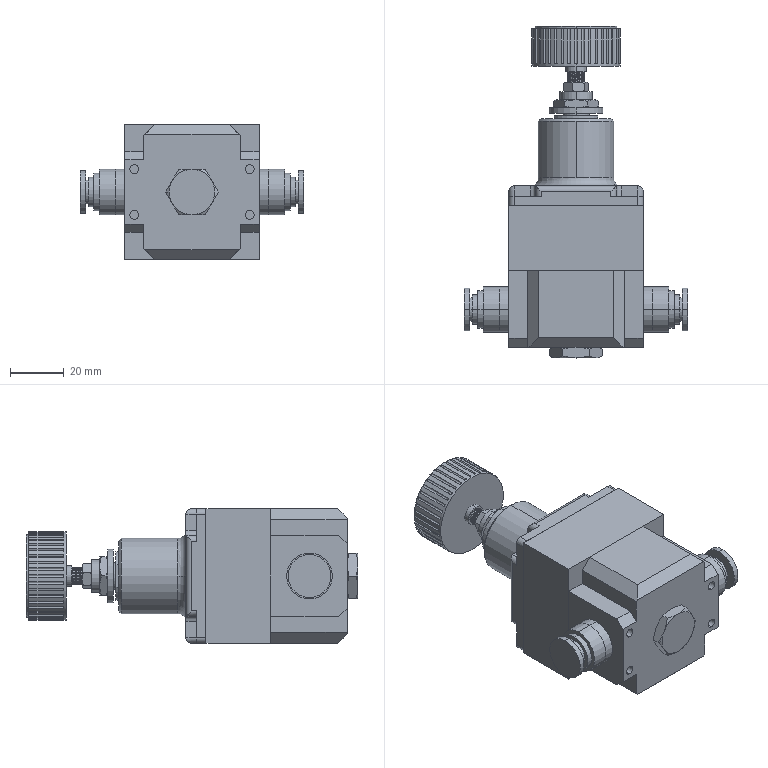Part | SolidWorks | features BaseBody 4 | 4 solids | 349 faces | box 83 x 123.4 x 50 mm | volume 174627 mm3 | cylinder 151 | plane 142 | cone 52 | spline 2 | torus 2 | commonest cylinder face diameters 0.887 x59 4 x20 6 x18 3.3 x8 7.9 x4 8.841 x4